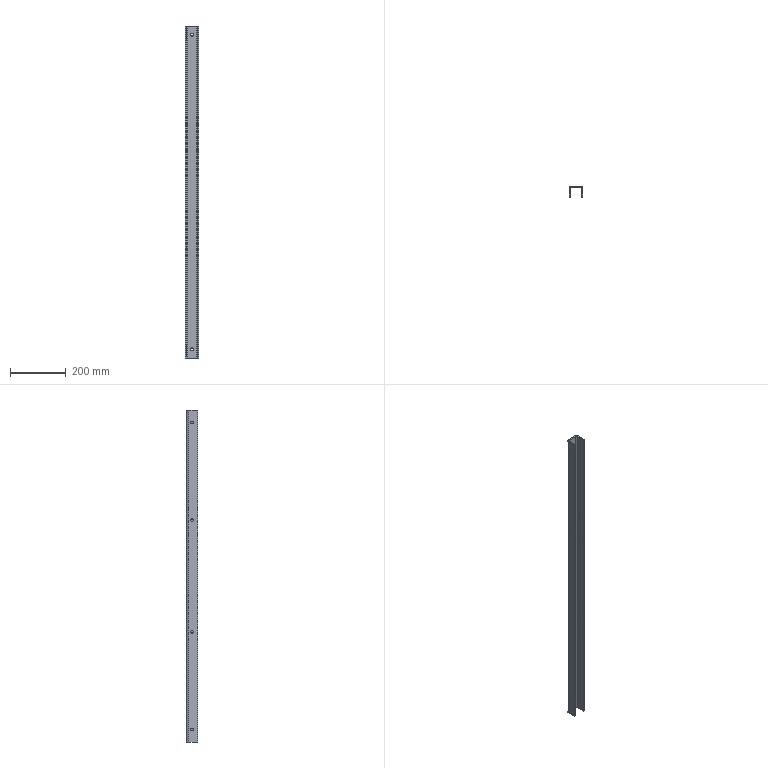Part | SolidWorks | features ICE 3, FlatPattern 1, SMBaseFlange 1, SheetMetal 1 | 1 solid | 42 faces | box 50 x 40 x 1190 mm | volume 552905 mm3 | cylinder 24 | plane 18 | commonest cylinder face diameters 11 x12 9 x8 8 x2 16 x2
STEP:
#1=CARTESIAN_POINT('',(-21.,-20.,554.5));
#2=VERTEX_POINT('',#1);
#3=CARTESIAN_POINT('',(-21.,-20.,545.5));
#4=VERTEX_POINT('',#3);
#5=CARTESIAN_POINT('',(-21.,-20.,550.));
#6=DIRECTION('',(1.,0.,0.));
#7=DIRECTION('',(0.,0.,1.));
#8=AXIS2_PLACEMENT_3D('',#5,#6,#7);
#9=CIRCLE('',#8,4.5);
#10=EDGE_CURVE('',#2,#4,#9,.T.);
#11=ORIENTED_EDGE('',*,*,#10,.T.);
#12=CARTESIAN_POINT('',(-25.,-20.,545.5));
#13=VERTEX_POINT('',#12);
#14=CARTESIAN_POINT('',(25.001,-20.,545.5));
#15=DIRECTION('',(-1.,0.,0.));
#16=VECTOR('',#15,1000.);
#17=LINE('',#14,#16);
#18=EDGE_CURVE('',#4,#13,#17,.T.);
#19=ORIENTED_EDGE('',*,*,#18,.T.);
#20=CARTESIAN_POINT('',(-25.,-20.,554.5));
#21=VERTEX_POINT('',#20);
#22=CARTESIAN_POINT('',(-25.,-20.,550.));
#23=DIRECTION('',(-1.,0.,0.));
#24=DIRECTION('',(0.,0.,1.));
#25=AXIS2_PLACEMENT_3D('',#22,#23,#24);
#26=CIRCLE('',#25,4.5);
#27=EDGE_CURVE('',#13,#21,#26,.T.);
#28=ORIENTED_EDGE('',*,*,#27,.T.);
#29=CARTESIAN_POINT('',(25.001,-20.,554.5));
#30=DIRECTION('',(-1.,0.,0.));
#31=VECTOR('',#30,1000.);
#32=LINE('',#29,#31);
#33=EDGE_CURVE('',#2,#21,#32,.T.);
#34=ORIENTED_EDGE('',*,*,#33,.F.);
#35=EDGE_LOOP('',(#11,#19,#28,#34));
#36=FACE_OUTER_BOUND('',#35,.T.);
#37=CARTESIAN_POINT('',(25.001,-20.,550.));
#38=DIRECTION('',(-1.,0.,0.));
#39=DIRECTION('',(0.,0.,1.));
#40=AXIS2_PLACEMENT_3D('',#37,#38,#39);
#41=CYLINDRICAL_SURFACE('',#40,4.5);
#42=ADVANCED_FACE('',(#36),#41,.F.);
#43=CARTESIAN_POINT('',(-21.,-20.,-545.5));
#44=VERTEX_POINT('',#43);
#45=CARTESIAN_POINT('',(-21.,-20.,-554.5));
#46=VERTEX_POINT('',#45);
#47=CARTESIAN_POINT('',(-21.,-20.,-550.));
#48=DIRECTION('',(1.,0.,0.));
#49=DIRECTION('',(0.,0.,1.));
#50=AXIS2_PLACEMENT_3D('',#47,#48,#49);
#51=CIRCLE('',#50,4.5);
#52=EDGE_CURVE('',#44,#46,#51,.T.);
#53=ORIENTED_EDGE('',*,*,#52,.T.);
#54=CARTESIAN_POINT('',(-25.,-20.,-554.5));
#55=VERTEX_POINT('',#54);
#56=CARTESIAN_POINT('',(25.001,-20.,-554.5));
#57=DIRECTION('',(-1.,0.,0.));
#58=VECTOR('',#57,1000.);
#59=LINE('',#56,#58);
#60=EDGE_CURVE('',#46,#55,#59,.T.);
#61=ORIENTED_EDGE('',*,*,#60,.T.);
#62=CARTESIAN_POINT('',(-25.,-20.,-545.5));
#63=VERTEX_POINT('',#62);
#64=CARTESIAN_POINT('',(-25.,-20.,-550.));
#65=DIRECTION('',(-1.,0.,0.));
#66=DIRECTION('',(0.,0.,-1.));
#67=AXIS2_PLACEMENT_3D('',#64,#65,#66);
#68=CIRCLE('',#67,4.5);
#69=EDGE_CURVE('',#55,#63,#68,.T.);
#70=ORIENTED_EDGE('',*,*,#69,.T.);
#71=CARTESIAN_POINT('',(25.001,-20.,-545.5));
#72=DIRECTION('',(-1.,0.,0.));
#73=VECTOR('',#72,1000.);
#74=LINE('',#71,#73);
#75=EDGE_CURVE('',#44,#63,#74,.T.);
#76=ORIENTED_EDGE('',*,*,#75,.F.);
#77=EDGE_LOOP('',(#53,#61,#70,#76));
#78=FACE_OUTER_BOUND('',#77,.T.);
#79=CARTESIAN_POINT('',(25.001,-20.,-550.));
#80=DIRECTION('',(-1.,0.,0.));
#81=DIRECTION('',(0.,0.,1.));
#82=AXIS2_PLACEMENT_3D('',#79,#80,#81);
#83=CYLINDRICAL_SURFACE('',#82,4.5);
#84=ADVANCED_FACE('',(#78),#83,.F.);
#85=CARTESIAN_POINT('',(-21.,-20.,-195.5));
#86=VERTEX_POINT('',#85);
#87=CARTESIAN_POINT('',(-21.,-20.,-204.5));
#88=VERTEX_POINT('',#87);
#89=CARTESIAN_POINT('',(-21.,-20.,-200.));
#90=DIRECTION('',(1.,0.,0.));
#91=DIRECTION('',(0.,0.,1.));
#92=AXIS2_PLACEMENT_3D('',#89,#90,#91);
#93=CIRCLE('',#92,4.5);
#94=EDGE_CURVE('',#86,#88,#93,.T.);
#95=ORIENTED_EDGE('',*,*,#94,.T.);
#96=CARTESIAN_POINT('',(-25.,-20.,-204.5));
#97=VERTEX_POINT('',#96);
#98=CARTESIAN_POINT('',(25.001,-20.,-204.5));
#99=DIRECTION('',(-1.,0.,0.));
#100=VECTOR('',#99,1000.);
#101=LINE('',#98,#100);
#102=EDGE_CURVE('',#88,#97,#101,.T.);
#103=ORIENTED_EDGE('',*,*,#102,.T.);
#104=CARTESIAN_POINT('',(-25.,-20.,-195.5));
#105=VERTEX_POINT('',#104);
#106=CARTESIAN_POINT('',(-25.,-20.,-200.));
#107=DIRECTION('',(-1.,0.,0.));
#108=DIRECTION('',(0.,0.,-1.));
#109=AXIS2_PLACEMENT_3D('',#106,#107,#108);
#110=CIRCLE('',#109,4.5);
#111=EDGE_CURVE('',#97,#105,#110,.T.);
#112=ORIENTED_EDGE('',*,*,#111,.T.);
#113=CARTESIAN_POINT('',(25.001,-20.,-195.5));
#114=DIRECTION('',(-1.,0.,0.));
#115=VECTOR('',#114,1000.);
#116=LINE('',#113,#115);
#117=EDGE_CURVE('',#86,#105,#116,.T.);
#118=ORIENTED_EDGE('',*,*,#117,.F.);
#119=EDGE_LOOP('',(#95,#103,#112,#118));
#120=FACE_OUTER_BOUND('',#119,.T.);
#121=CARTESIAN_POINT('',(25.001,-20.,-200.));
#122=DIRECTION('',(-1.,0.,0.));
#123=DIRECTION('',(0.,0.,1.));
#124=AXIS2_PLACEMENT_3D('',#121,#122,#123);
#125=CYLINDRICAL_SURFACE('',#124,4.5);
#126=ADVANCED_FACE('',(#120),#125,.F.);
#127=CARTESIAN_POINT('',(-21.,-20.,204.5));
#128=VERTEX_POINT('',#127);
#129=CARTESIAN_POINT('',(-21.,-20.,195.5));
#130=VERTEX_POINT('',#129);
#131=CARTESIAN_POINT('',(-21.,-20.,200.));
#132=DIRECTION('',(1.,0.,0.));
#133=DIRECTION('',(0.,0.,1.));
#134=AXIS2_PLACEMENT_3D('',#131,#132,#133);
#135=CIRCLE('',#134,4.5);
#136=EDGE_CURVE('',#128,#130,#135,.T.);
#137=ORIENTED_EDGE('',*,*,#136,.T.);
#138=CARTESIAN_POINT('',(-25.,-20.,195.5));
#139=VERTEX_POINT('',#138);
#140=CARTESIAN_POINT('',(25.001,-20.,195.5));
#141=DIRECTION('',(-1.,0.,0.));
#142=VECTOR('',#141,1000.);
#143=LINE('',#140,#142);
#144=EDGE_CURVE('',#130,#139,#143,.T.);
#145=ORIENTED_EDGE('',*,*,#144,.T.);
#146=CARTESIAN_POINT('',(-25.,-20.,204.5));
#147=VERTEX_POINT('',#146);
#148=CARTESIAN_POINT('',(-25.,-20.,200.));
#149=DIRECTION('',(-1.,0.,0.));
#150=DIRECTION('',(0.,0.,1.));
#151=AXIS2_PLACEMENT_3D('',#148,#149,#150);
#152=CIRCLE('',#151,4.5);
#153=EDGE_CURVE('',#139,#147,#152,.T.);
#154=ORIENTED_EDGE('',*,*,#153,.T.);
#155=CARTESIAN_POINT('',(25.001,-20.,204.5));
#156=DIRECTION('',(-1.,0.,0.));
#157=VECTOR('',#156,1000.);
#158=LINE('',#155,#157);
#159=EDGE_CURVE('',#128,#147,#158,.T.);
#160=ORIENTED_EDGE('',*,*,#159,.F.);
#161=EDGE_LOOP('',(#137,#145,#154,#160));
#162=FACE_OUTER_BOUND('',#161,.T.);
#163=CARTESIAN_POINT('',(25.001,-20.,200.));
#164=DIRECTION('',(-1.,0.,0.));
#165=DIRECTION('',(0.,0.,1.));
#166=AXIS2_PLACEMENT_3D('',#163,#164,#165);
#167=CYLINDRICAL_SURFACE('',#166,4.5);
#168=ADVANCED_FACE('',(#162),#167,.F.);
#169=CARTESIAN_POINT('',(21.,-20.,252.));
#170=VERTEX_POINT('',#169);
#171=CARTESIAN_POINT('',(21.,-20.,263.));
#172=VERTEX_POINT('',#171);
#173=CARTESIAN_POINT('',(21.,-20.,257.5));
#174=DIRECTION('',(-1.,0.,0.));
#175=DIRECTION('',(0.,0.,-1.));
#176=AXIS2_PLACEMENT_3D('',#173,#174,#175);
#177=CIRCLE('',#176,5.5);
#178=EDGE_CURVE('',#170,#172,#177,.T.);
#179=ORIENTED_EDGE('',*,*,#178,.T.);
#180=CARTESIAN_POINT('',(25.,-20.,263.));
#181=VERTEX_POINT('',#180);
#182=CARTESIAN_POINT('',(-25.001,-20.,263.));
#183=DIRECTION('',(1.,0.,0.));
#184=VECTOR('',#183,1000.);
#185=LINE('',#182,#184);
#186=EDGE_CURVE('',#172,#181,#185,.T.);
#187=ORIENTED_EDGE('',*,*,#186,.T.);
#188=CARTESIAN_POINT('',(25.,-20.,252.));
#189=VERTEX_POINT('',#188);
#190=CARTESIAN_POINT('',(25.,-20.,257.5));
#191=DIRECTION('',(1.,0.,0.));
#192=DIRECTION('',(0.,0.,-1.));
#193=AXIS2_PLACEMENT_3D('',#190,#191,#192);
#194=CIRCLE('',#193,5.5);
#195=EDGE_CURVE('',#181,#189,#194,.T.);
#196=ORIENTED_EDGE('',*,*,#195,.T.);
#197=CARTESIAN_POINT('',(-25.001,-20.,252.));
#198=DIRECTION('',(1.,0.,0.));
#199=VECTOR('',#198,1000.);
#200=LINE('',#197,#199);
#201=EDGE_CURVE('',#170,#189,#200,.T.);
#202=ORIENTED_EDGE('',*,*,#201,.F.);
#203=EDGE_LOOP('',(#179,#187,#196,#202));
#204=FACE_OUTER_BOUND('',#203,.T.);
#205=CARTESIAN_POINT('',(-25.001,-20.,257.5));
#206=DIRECTION('',(1.,0.,0.));
#207=DIRECTION('',(0.,0.,-1.));
#208=AXIS2_PLACEMENT_3D('',#205,#206,#207);
#209=CYLINDRICAL_SURFACE('',#208,5.5);
#210=ADVANCED_FACE('',(#204),#209,.F.);
#211=CARTESIAN_POINT('',(21.,-20.,147.));
#212=VERTEX_POINT('',#211);
#213=CARTESIAN_POINT('',(21.,-20.,158.));
#214=VERTEX_POINT('',#213);
#215=CARTESIAN_POINT('',(21.,-20.,152.5));
#216=DIRECTION('',(-1.,0.,0.));
#217=DIRECTION('',(0.,0.,-1.));
#218=AXIS2_PLACEMENT_3D('',#215,#216,#217);
#219=CIRCLE('',#218,5.5);
#220=EDGE_CURVE('',#212,#214,#219,.T.);
#221=ORIENTED_EDGE('',*,*,#220,.T.);
#222=CARTESIAN_POINT('',(25.,-20.,158.));
#223=VERTEX_POINT('',#222);
#224=CARTESIAN_POINT('',(-25.001,-20.,158.));
#225=DIRECTION('',(1.,0.,0.));
#226=VECTOR('',#225,1000.);
#227=LINE('',#224,#226);
#228=EDGE_CURVE('',#214,#223,#227,.T.);
#229=ORIENTED_EDGE('',*,*,#228,.T.);
#230=CARTESIAN_POINT('',(25.,-20.,147.));
#231=VERTEX_POINT('',#230);
#232=CARTESIAN_POINT('',(25.,-20.,152.5));
#233=DIRECTION('',(1.,0.,0.));
#234=DIRECTION('',(0.,0.,-1.));
#235=AXIS2_PLACEMENT_3D('',#232,#233,#234);
#236=CIRCLE('',#235,5.5);
#237=EDGE_CURVE('',#223,#231,#236,.T.);
#238=ORIENTED_EDGE('',*,*,#237,.T.);
#239=CARTESIAN_POINT('',(-25.001,-20.,147.));
#240=DIRECTION('',(1.,0.,0.));
#241=VECTOR('',#240,1000.);
#242=LINE('',#239,#241);
#243=EDGE_CURVE('',#212,#231,#242,.T.);
#244=ORIENTED_EDGE('',*,*,#243,.F.);
#245=EDGE_LOOP('',(#221,#229,#238,#244));
#246=FACE_OUTER_BOUND('',#245,.T.);
#247=CARTESIAN_POINT('',(-25.001,-20.,152.5));
#248=DIRECTION('',(1.,0.,0.));
#249=DIRECTION('',(0.,0.,-1.));
#250=AXIS2_PLACEMENT_3D('',#247,#248,#249);
#251=CYLINDRICAL_SURFACE('',#250,5.5);
#252=ADVANCED_FACE('',(#246),#251,.F.);
#253=CARTESIAN_POINT('',(21.,-20.,-158.));
#254=VERTEX_POINT('',#253);
#255=CARTESIAN_POINT('',(21.,-20.,-147.));
#256=VERTEX_POINT('',#255);
#257=CARTESIAN_POINT('',(21.,-20.,-152.5));
#258=DIRECTION('',(-1.,0.,0.));
#259=DIRECTION('',(0.,0.,-1.));
#260=AXIS2_PLACEMENT_3D('',#257,#258,#259);
#261=CIRCLE('',#260,5.5);
#262=EDGE_CURVE('',#254,#256,#261,.T.);
#263=ORIENTED_EDGE('',*,*,#262,.T.);
#264=CARTESIAN_POINT('',(25.,-20.,-147.));
#265=VERTEX_POINT('',#264);
#266=CARTESIAN_POINT('',(-25.001,-20.,-147.));
#267=DIRECTION('',(1.,0.,0.));
#268=VECTOR('',#267,1000.);
#269=LINE('',#266,#268);
#270=EDGE_CURVE('',#256,#265,#269,.T.);
#271=ORIENTED_EDGE('',*,*,#270,.T.);
#272=CARTESIAN_POINT('',(25.,-20.,-158.));
#273=VERTEX_POINT('',#272);
#274=CARTESIAN_POINT('',(25.,-20.,-152.5));
#275=DIRECTION('',(1.,0.,0.));
#276=DIRECTION('',(0.,0.,1.));
#277=AXIS2_PLACEMENT_3D('',#274,#275,#276);
#278=CIRCLE('',#277,5.5);
#279=EDGE_CURVE('',#265,#273,#278,.T.);
#280=ORIENTED_EDGE('',*,*,#279,.T.);
#281=CARTESIAN_POINT('',(-25.001,-20.,-158.));
#282=DIRECTION('',(1.,0.,0.));
#283=VECTOR('',#282,1000.);
#284=LINE('',#281,#283);
#285=EDGE_CURVE('',#254,#273,#284,.T.);
#286=ORIENTED_EDGE('',*,*,#285,.F.);
#287=EDGE_LOOP('',(#263,#271,#280,#286));
#288=FACE_OUTER_BOUND('',#287,.T.);
#289=CARTESIAN_POINT('',(-25.001,-20.,-152.5));
#290=DIRECTION('',(1.,0.,0.));
#291=DIRECTION('',(0.,0.,-1.));
#292=AXIS2_PLACEMENT_3D('',#289,#290,#291);
#293=CYLINDRICAL_SURFACE('',#292,5.5);
#294=ADVANCED_FACE('',(#288),#293,.F.);
#295=CARTESIAN_POINT('',(21.,-20.,-263.));
#296=VERTEX_POINT('',#295);
#297=CARTESIAN_POINT('',(21.,-20.,-252.));
#298=VERTEX_POINT('',#297);
#299=CARTESIAN_POINT('',(21.,-20.,-257.5));
#300=DIRECTION('',(-1.,0.,0.));
#301=DIRECTION('',(0.,0.,-1.));
#302=AXIS2_PLACEMENT_3D('',#299,#300,#301);
#303=CIRCLE('',#302,5.5);
#304=EDGE_CURVE('',#296,#298,#303,.T.);
#305=ORIENTED_EDGE('',*,*,#304,.T.);
#306=CARTESIAN_POINT('',(25.,-20.,-252.));
#307=VERTEX_POINT('',#306);
#308=CARTESIAN_POINT('',(-25.001,-20.,-252.));
#309=DIRECTION('',(1.,0.,0.));
#310=VECTOR('',#309,1000.);
#311=LINE('',#308,#310);
#312=EDGE_CURVE('',#298,#307,#311,.T.);
#313=ORIENTED_EDGE('',*,*,#312,.T.);
#314=CARTESIAN_POINT('',(25.,-20.,-263.));
#315=VERTEX_POINT('',#314);
#316=CARTESIAN_POINT('',(25.,-20.,-257.5));
#317=DIRECTION('',(1.,0.,0.));
#318=DIRECTION('',(0.,0.,1.));
#319=AXIS2_PLACEMENT_3D('',#316,#317,#318);
#320=CIRCLE('',#319,5.5);
#321=EDGE_CURVE('',#307,#315,#320,.T.);
#322=ORIENTED_EDGE('',*,*,#321,.T.);
#323=CARTESIAN_POINT('',(-25.001,-20.,-263.));
#324=DIRECTION('',(1.,0.,0.));
#325=VECTOR('',#324,1000.);
#326=LINE('',#323,#325);
#327=EDGE_CURVE('',#296,#315,#326,.T.);
#328=ORIENTED_EDGE('',*,*,#327,.F.);
#329=EDGE_LOOP('',(#305,#313,#322,#328));
#330=FACE_OUTER_BOUND('',#329,.T.);
#331=CARTESIAN_POINT('',(-25.001,-20.,-257.5));
#332=DIRECTION('',(1.,0.,0.));
#333=DIRECTION('',(0.,0.,-1.));
#334=AXIS2_PLACEMENT_3D('',#331,#332,#333);
#335=CYLINDRICAL_SURFACE('',#334,5.5);
#336=ADVANCED_FACE('',(#330),#335,.F.);
#337=CARTESIAN_POINT('',(5.5,-4.,564.));
#338=VERTEX_POINT('',#337);
#339=CARTESIAN_POINT('',(-5.5,-4.,564.));
#340=VERTEX_POINT('',#339);
#341=CARTESIAN_POINT('',(0.,-4.,564.));
#342=DIRECTION('',(0.,1.,0.));
#343=DIRECTION('',(0.,0.,1.));
#344=AXIS2_PLACEMENT_3D('',#341,#342,#343);
#345=CIRCLE('',#344,5.5);
#346=EDGE_CURVE('',#338,#340,#345,.T.);
#347=ORIENTED_EDGE('',*,*,#346,.F.);
#348=CARTESIAN_POINT('',(5.5,0.,564.));
#349=VERTEX_POINT('',#348);
#350=CARTESIAN_POINT('',(5.5,-40.,564.));
#351=DIRECTION('',(0.,1.,0.));
#352=VECTOR('',#351,1000.);
#353=LINE('',#350,#352);
#354=EDGE_CURVE('',#338,#349,#353,.T.);
#355=ORIENTED_EDGE('',*,*,#354,.T.);
#356=CARTESIAN_POINT('',(-5.5,0.,564.));
#357=VERTEX_POINT('',#356);
#358=CARTESIAN_POINT('',(0.,0.,564.));
#359=DIRECTION('',(0.,1.,0.));
#360=DIRECTION('',(-1.,0.,0.));
#361=AXIS2_PLACEMENT_3D('',#358,#359,#360);
#362=CIRCLE('',#361,5.5);
#363=EDGE_CURVE('',#349,#357,#362,.T.);
#364=ORIENTED_EDGE('',*,*,#363,.T.);
#365=CARTESIAN_POINT('',(-5.5,-40.,564.));
#366=DIRECTION('',(0.,1.,0.));
#367=VECTOR('',#366,1000.);
#368=LINE('',#365,#367);
#369=EDGE_CURVE('',#340,#357,#368,.T.);
#370=ORIENTED_EDGE('',*,*,#369,.F.);
#371=EDGE_LOOP('',(#347,#355,#364,#370));
#372=FACE_OUTER_BOUND('',#371,.T.);
#373=CARTESIAN_POINT('',(0.,-40.,564.));
#374=DIRECTION('',(0.,1.,0.));
#375=DIRECTION('',(-1.,0.,0.));
#376=AXIS2_PLACEMENT_3D('',#373,#374,#375);
#377=CYLINDRICAL_SURFACE('',#376,5.5);
#378=ADVANCED_FACE('',(#372),#377,.F.);
#379=CARTESIAN_POINT('',(5.5,-4.,-564.));
#380=VERTEX_POINT('',#379);
#381=CARTESIAN_POINT('',(-5.5,-4.,-564.));
#382=VERTEX_POINT('',#381);
#383=CARTESIAN_POINT('',(0.,-4.,-564.));
#384=DIRECTION('',(0.,1.,0.));
#385=DIRECTION('',(0.,0.,1.));
#386=AXIS2_PLACEMENT_3D('',#383,#384,#385);
#387=CIRCLE('',#386,5.5);
#388=EDGE_CURVE('',#380,#382,#387,.T.);
#389=ORIENTED_EDGE('',*,*,#388,.F.);
#390=CARTESIAN_POINT('',(5.5,0.,-564.));
#391=VERTEX_POINT('',#390);
#392=CARTESIAN_POINT('',(5.5,-40.,-564.));
#393=DIRECTION('',(0.,1.,0.));
#394=VECTOR('',#393,1000.);
#395=LINE('',#392,#394);
#396=EDGE_CURVE('',#380,#391,#395,.T.);
#397=ORIENTED_EDGE('',*,*,#396,.T.);
#398=CARTESIAN_POINT('',(-5.5,0.,-564.));
#399=VERTEX_POINT('',#398);
#400=CARTESIAN_POINT('',(0.,0.,-564.));
#401=DIRECTION('',(0.,1.,0.));
#402=DIRECTION('',(1.,0.,0.));
#403=AXIS2_PLACEMENT_3D('',#400,#401,#402);
#404=CIRCLE('',#403,5.5);
#405=EDGE_CURVE('',#391,#399,#404,.T.);
#406=ORIENTED_EDGE('',*,*,#405,.T.);
#407=CARTESIAN_POINT('',(-5.5,-40.,-564.));
#408=DIRECTION('',(0.,1.,0.));
#409=VECTOR('',#408,1000.);
#410=LINE('',#407,#409);
#411=EDGE_CURVE('',#382,#399,#410,.T.);
#412=ORIENTED_EDGE('',*,*,#411,.F.);
#413=EDGE_LOOP('',(#389,#397,#406,#412));
#414=FACE_OUTER_BOUND('',#413,.T.);
#415=CARTESIAN_POINT('',(0.,-40.,-564.));
#416=DIRECTION('',(0.,1.,0.));
#417=DIRECTION('',(-1.,0.,0.));
#418=AXIS2_PLACEMENT_3D('',#415,#416,#417);
#419=CYLINDRICAL_SURFACE('',#418,5.5);
#420=ADVANCED_FACE('',(#414),#419,.F.);
#421=CARTESIAN_POINT('',(-17.,0.,595.));
#422=VERTEX_POINT('',#421);
#423=CARTESIAN_POINT('',(-17.,-4.,595.));
#424=VERTEX_POINT('',#423);
#425=CARTESIAN_POINT('',(-17.,0.,595.));
#426=DIRECTION('',(0.,-1.,0.));
#427=VECTOR('',#426,1000.);
#428=LINE('',#425,#427);
#429=EDGE_CURVE('',#422,#424,#428,.T.);
#430=ORIENTED_EDGE('',*,*,#429,.F.);
#431=CARTESIAN_POINT('',(-25.,-8.,595.));
#432=VERTEX_POINT('',#431);
#433=CARTESIAN_POINT('',(-17.,-8.,595.));
#434=DIRECTION('',(0.,0.,-1.));
#435=DIRECTION('',(1.,0.,0.));
#436=AXIS2_PLACEMENT_3D('',#433,#434,#435);
#437=CIRCLE('',#436,8.);
#438=EDGE_CURVE('',#432,#422,#437,.T.);
#439=ORIENTED_EDGE('',*,*,#438,.F.);
#440=CARTESIAN_POINT('',(-21.,-8.,595.));
#441=VERTEX_POINT('',#440);
#442=CARTESIAN_POINT('',(-21.,-8.,595.));
#443=DIRECTION('',(-1.,0.,0.));
#444=VECTOR('',#443,1000.);
#445=LINE('',#442,#444);
#446=EDGE_CURVE('',#441,#432,#445,.T.);
#447=ORIENTED_EDGE('',*,*,#446,.F.);
#448=CARTESIAN_POINT('',(-17.,-8.,595.));
#449=DIRECTION('',(0.,0.,-1.));
#450=DIRECTION('',(1.,0.,0.));
#451=AXIS2_PLACEMENT_3D('',#448,#449,#450);
#452=CIRCLE('',#451,4.);
#453=EDGE_CURVE('',#441,#424,#452,.T.);
#454=ORIENTED_EDGE('',*,*,#453,.T.);
#455=EDGE_LOOP('',(#430,#439,#447,#454));
#456=FACE_OUTER_BOUND('',#455,.T.);
#457=CARTESIAN_POINT('',(-17.,0.,595.));
#458=DIRECTION('',(0.,0.,1.));
#459=DIRECTION('',(1.,0.,0.));
#460=AXIS2_PLACEMENT_3D('',#457,#458,#459);
#461=PLANE('',#460);
#462=ADVANCED_FACE('',(#456),#461,.T.);
#463=CARTESIAN_POINT('',(17.,0.,595.));
#464=VERTEX_POINT('',#463);
#465=CARTESIAN_POINT('',(-25.,0.,595.));
#466=DIRECTION('',(1.,0.,0.));
#467=VECTOR('',#466,1000.);
#468=LINE('',#465,#467);
#469=EDGE_CURVE('',#422,#464,#468,.T.);
#470=ORIENTED_EDGE('',*,*,#469,.F.);
#471=ORIENTED_EDGE('',*,*,#429,.T.);
#472=CARTESIAN_POINT('',(17.,-4.,595.));
#473=VERTEX_POINT('',#472);
#474=CARTESIAN_POINT('',(-25.,-4.,595.));
#475=DIRECTION('',(1.,0.,0.));
#476=VECTOR('',#475,1000.);
#477=LINE('',#474,#476);
#478=EDGE_CURVE('',#424,#473,#477,.T.);
#479=ORIENTED_EDGE('',*,*,#478,.T.);
#480=CARTESIAN_POINT('',(17.,-4.,595.));
#481=DIRECTION('',(0.,1.,0.));
#482=VECTOR('',#481,1000.);
#483=LINE('',#480,#482);
#484=EDGE_CURVE('',#473,#464,#483,.T.);
#485=ORIENTED_EDGE('',*,*,#484,.T.);
#486=EDGE_LOOP('',(#470,#471,#479,#485));
#487=FACE_OUTER_BOUND('',#486,.T.);
#488=CARTESIAN_POINT('',(-21.,-8.,595.));
#489=DIRECTION('',(0.,0.,1.));
#490=DIRECTION('',(1.,0.,0.));
#491=AXIS2_PLACEMENT_3D('',#488,#489,#490);
#492=PLANE('',#491);
#493=ADVANCED_FACE('',(#487),#492,.T.);
#494=CARTESIAN_POINT('',(-25.,-8.,-595.));
#495=VERTEX_POINT('',#494);
#496=CARTESIAN_POINT('',(-21.,-8.,-595.));
#497=VERTEX_POINT('',#496);
#498=CARTESIAN_POINT('',(-25.,-8.,-595.));
#499=DIRECTION('',(1.,0.,0.));
#500=VECTOR('',#499,1000.);
#501=LINE('',#498,#500);
#502=EDGE_CURVE('',#495,#497,#501,.T.);
#503=ORIENTED_EDGE('',*,*,#502,.F.);
#504=CARTESIAN_POINT('',(-17.,0.,-595.));
#505=VERTEX_POINT('',#504);
#506=CARTESIAN_POINT('',(-17.,-8.,-595.));
#507=DIRECTION('',(0.,0.,-1.));
#508=DIRECTION('',(1.,0.,0.));
#509=AXIS2_PLACEMENT_3D('',#506,#507,#508);
#510=CIRCLE('',#509,8.);
#511=EDGE_CURVE('',#495,#505,#510,.T.);
#512=ORIENTED_EDGE('',*,*,#511,.T.);
#513=CARTESIAN_POINT('',(-17.,-4.,-595.));
#514=VERTEX_POINT('',#513);
#515=CARTESIAN_POINT('',(-17.,-4.,-595.));
#516=DIRECTION('',(0.,1.,0.));
#517=VECTOR('',#516,1000.);
#518=LINE('',#515,#517);
#519=EDGE_CURVE('',#514,#505,#518,.T.);
#520=ORIENTED_EDGE('',*,*,#519,.F.);
#521=CARTESIAN_POINT('',(-17.,-8.,-595.));
#522=DIRECTION('',(0.,0.,-1.));
#523=DIRECTION('',(1.,0.,0.));
#524=AXIS2_PLACEMENT_3D('',#521,#522,#523);
#525=CIRCLE('',#524,4.);
#526=EDGE_CURVE('',#497,#514,#525,.T.);
#527=ORIENTED_EDGE('',*,*,#526,.F.);
#528=EDGE_LOOP('',(#503,#512,#520,#527));
#529=FACE_OUTER_BOUND('',#528,.T.);
#530=CARTESIAN_POINT('',(-25.,-8.,-595.));
#531=DIRECTION('',(0.,0.,-1.));
#532=DIRECTION('',(-1.,0.,0.));
#533=AXIS2_PLACEMENT_3D('',#530,#531,#532);
#534=PLANE('',#533);
#535=ADVANCED_FACE('',(#529),#534,.T.);
#536=CARTESIAN_POINT('',(-25.,-40.,-595.));
#537=VERTEX_POINT('',#536);
#538=CARTESIAN_POINT('',(-25.,-40.,-595.));
#539=DIRECTION('',(0.,1.,0.));
#540=VECTOR('',#539,1000.);
#541=LINE('',#538,#540);
#542=EDGE_CURVE('',#537,#495,#541,.T.);
#543=ORIENTED_EDGE('',*,*,#542,.T.);
#544=ORIENTED_EDGE('',*,*,#502,.T.);
#545=CARTESIAN_POINT('',(-21.,-40.,-595.));
#546=VERTEX_POINT('',#545);
#547=CARTESIAN_POINT('',(-21.,-40.,-595.));
#548=DIRECTION('',(0.,1.,0.));
#549=VECTOR('',#548,1000.);
#550=LINE('',#547,#549);
#551=EDGE_CURVE('',#546,#497,#550,.T.);
#552=ORIENTED_EDGE('',*,*,#551,.F.);
#553=CARTESIAN_POINT('',(-21.,-40.,-595.));
#554=DIRECTION('',(-1.,0.,0.));
#555=VECTOR('',#554,1000.);
#556=LINE('',#553,#555);
#557=EDGE_CURVE('',#546,#537,#556,.T.);
#558=ORIENTED_EDGE('',*,*,#557,.T.);
#559=EDGE_LOOP('',(#543,#544,#552,#558));
#560=FACE_OUTER_BOUND('',#559,.T.);
#561=CARTESIAN_POINT('',(-17.,-4.,-595.));
#562=DIRECTION('',(0.,0.,-1.));
#563=DIRECTION('',(-1.,0.,0.));
#564=AXIS2_PLACEMENT_3D('',#561,#562,#563);
#565=PLANE('',#564);
#566=ADVANCED_FACE('',(#560),#565,.T.);
#567=CARTESIAN_POINT('',(25.,-8.,595.));
#568=VERTEX_POINT('',#567);
#569=CARTESIAN_POINT('',(21.,-8.,595.));
#570=VERTEX_POINT('',#569);
#571=CARTESIAN_POINT('',(25.,-8.,595.));
#572=DIRECTION('',(-1.,0.,0.));
#573=VECTOR('',#572,1000.);
#574=LINE('',#571,#573);
#575=EDGE_CURVE('',#568,#570,#574,.T.);
#576=ORIENTED_EDGE('',*,*,#575,.F.);
#577=CARTESIAN_POINT('',(17.,-8.,595.));
#578=DIRECTION('',(0.,0.,-1.));
#579=DIRECTION('',(1.,0.,0.));
#580=AXIS2_PLACEMENT_3D('',#577,#578,#579);
#581=CIRCLE('',#580,8.);
#582=EDGE_CURVE('',#464,#568,#581,.T.);
#583=ORIENTED_EDGE('',*,*,#582,.F.);
#584=ORIENTED_EDGE('',*,*,#484,.F.);
#585=CARTESIAN_POINT('',(17.,-8.,595.));
#586=DIRECTION('',(0.,0.,-1.));
#587=DIRECTION('',(1.,0.,0.));
#588=AXIS2_PLACEMENT_3D('',#585,#586,#587);
#589=CIRCLE('',#588,4.);
#590=EDGE_CURVE('',#473,#570,#589,.T.);
#591=ORIENTED_EDGE('',*,*,#590,.T.);
#592=EDGE_LOOP('',(#576,#583,#584,#591));
#593=FACE_OUTER_BOUND('',#592,.T.);
#594=CARTESIAN_POINT('',(25.,-8.,595.));
#595=DIRECTION('',(0.,0.,1.));
#596=DIRECTION('',(1.,0.,0.));
#597=AXIS2_PLACEMENT_3D('',#594,#595,#596);
#598=PLANE('',#597);
#599=ADVANCED_FACE('',(#593),#598,.T.);
#600=CARTESIAN_POINT('',(25.,-40.,595.));
#601=VERTEX_POINT('',#600);
#602=CARTESIAN_POINT('',(25.,0.,595.));
#603=DIRECTION('',(0.,-1.,0.));
#604=VECTOR('',#603,1000.);
#605=LINE('',#602,#604);
#606=EDGE_CURVE('',#568,#601,#605,.T.);
#607=ORIENTED_EDGE('',*,*,#606,.F.);
#608=ORIENTED_EDGE('',*,*,#575,.T.);
#609=CARTESIAN_POINT('',(21.,-40.,595.));
#610=VERTEX_POINT('',#609);
#611=CARTESIAN_POINT('',(21.,0.,595.));
#612=DIRECTION('',(0.,-1.,0.));
#613=VECTOR('',#612,1000.);
#614=LINE('',#611,#613);
#615=EDGE_CURVE('',#570,#610,#614,.T.);
#616=ORIENTED_EDGE('',*,*,#615,.T.);
#617=CARTESIAN_POINT('',(25.,-40.,595.));
#618=DIRECTION('',(-1.,0.,0.));
#619=VECTOR('',#618,1000.);
#620=LINE('',#617,#619);
#621=EDGE_CURVE('',#601,#610,#620,.T.);
#622=ORIENTED_EDGE('',*,*,#621,.F.);
#623=EDGE_LOOP('',(#607,#608,#616,#622));
#624=FACE_OUTER_BOUND('',#623,.T.);
#625=CARTESIAN_POINT('',(17.,-4.,595.));
#626=DIRECTION('',(0.,0.,1.));
#627=DIRECTION('',(1.,0.,0.));
#628=AXIS2_PLACEMENT_3D('',#625,#626,#627);
#629=PLANE('',#628);
#630=ADVANCED_FACE('',(#624),#629,.T.);
#631=CARTESIAN_POINT('',(17.,0.,-595.));
#632=VERTEX_POINT('',#631);
#633=CARTESIAN_POINT('',(17.,-4.,-595.));
#634=VERTEX_POINT('',#633);
#635=CARTESIAN_POINT('',(17.,0.,-595.));
#636=DIRECTION('',(0.,-1.,0.));
#637=VECTOR('',#636,1000.);
#638=LINE('',#635,#637);
#639=EDGE_CURVE('',#632,#634,#638,.T.);
#640=ORIENTED_EDGE('',*,*,#639,.F.);
#641=CARTESIAN_POINT('',(25.,-8.,-595.));
#642=VERTEX_POINT('',#641);
#643=CARTESIAN_POINT('',(17.,-8.,-595.));
#644=DIRECTION('',(0.,0.,-1.));
#645=DIRECTION('',(1.,0.,0.));
#646=AXIS2_PLACEMENT_3D('',#643,#644,#645);
#647=CIRCLE('',#646,8.);
#648=EDGE_CURVE('',#632,#642,#647,.T.);
#649=ORIENTED_EDGE('',*,*,#648,.T.);
#650=CARTESIAN_POINT('',(21.,-8.,-595.));
#651=VERTEX_POINT('',#650);
#652=CARTESIAN_POINT('',(21.,-8.,-595.));
#653=DIRECTION('',(1.,0.,0.));
#654=VECTOR('',#653,1000.);
#655=LINE('',#652,#654);
#656=EDGE_CURVE('',#651,#642,#655,.T.);
#657=ORIENTED_EDGE('',*,*,#656,.F.);
#658=CARTESIAN_POINT('',(17.,-8.,-595.));
#659=DIRECTION('',(0.,0.,-1.));
#660=DIRECTION('',(1.,0.,0.));
#661=AXIS2_PLACEMENT_3D('',#658,#659,#660);
#662=CIRCLE('',#661,4.);
#663=EDGE_CURVE('',#634,#651,#662,.T.);
#664=ORIENTED_EDGE('',*,*,#663,.F.);
#665=EDGE_LOOP('',(#640,#649,#657,#664));
#666=FACE_OUTER_BOUND('',#665,.T.);
#667=CARTESIAN_POINT('',(17.,0.,-595.));
#668=DIRECTION('',(0.,0.,-1.));
#669=DIRECTION('',(-1.,0.,0.));
#670=AXIS2_PLACEMENT_3D('',#667,#668,#669);
#671=PLANE('',#670);
#672=ADVANCED_FACE('',(#666),#671,.T.);
#673=CARTESIAN_POINT('',(-25.,0.,-595.));
#674=DIRECTION('',(1.,0.,0.));
#675=VECTOR('',#674,1000.);
#676=LINE('',#673,#675);
#677=EDGE_CURVE('',#505,#632,#676,.T.);
#678=ORIENTED_EDGE('',*,*,#677,.T.);
#679=ORIENTED_EDGE('',*,*,#639,.T.);
#680=CARTESIAN_POINT('',(-25.,-4.,-595.));
#681=DIRECTION('',(1.,0.,0.));
#682=VECTOR('',#681,1000.);
#683=LINE('',#680,#682);
#684=EDGE_CURVE('',#514,#634,#683,.T.);
#685=ORIENTED_EDGE('',*,*,#684,.F.);
#686=ORIENTED_EDGE('',*,*,#519,.T.);
#687=EDGE_LOOP('',(#678,#679,#685,#686));
#688=FACE_OUTER_BOUND('',#687,.T.);
#689=CARTESIAN_POINT('',(21.,-8.,-595.));
#690=DIRECTION('',(0.,0.,-1.));
#691=DIRECTION('',(-1.,0.,0.));
#692=AXIS2_PLACEMENT_3D('',#689,#690,#691);
#693=PLANE('',#692);
#694=ADVANCED_FACE('',(#688),#693,.T.);
#695=ORIENTED_EDGE('',*,*,#178,.F.);
#696=CARTESIAN_POINT('',(21.,-20.,257.5));
#697=DIRECTION('',(-1.,0.,0.));
#698=DIRECTION('',(0.,0.,-1.));
#699=AXIS2_PLACEMENT_3D('',#696,#697,#698);
#700=CIRCLE('',#699,5.5);
#701=EDGE_CURVE('',#172,#170,#700,.T.);
#702=ORIENTED_EDGE('',*,*,#701,.F.);
#703=EDGE_LOOP('',(#695,#702));
#704=FACE_BOUND('',#703,.T.);
#705=ORIENTED_EDGE('',*,*,#220,.F.);
#706=CARTESIAN_POINT('',(21.,-20.,152.5));
#707=DIRECTION('',(-1.,0.,0.));
#708=DIRECTION('',(0.,0.,-1.));
#709=AXIS2_PLACEMENT_3D('',#706,#707,#708);
#710=CIRCLE('',#709,5.5);
#711=EDGE_CURVE('',#214,#212,#710,.T.);
#712=ORIENTED_EDGE('',*,*,#711,.F.);
#713=EDGE_LOOP('',(#705,#712));
#714=FACE_BOUND('',#713,.T.);
#715=ORIENTED_EDGE('',*,*,#262,.F.);
#716=CARTESIAN_POINT('',(21.,-20.,-152.5));
#717=DIRECTION('',(-1.,0.,0.));
#718=DIRECTION('',(0.,0.,-1.));
#719=AXIS2_PLACEMENT_3D('',#716,#717,#718);
#720=CIRCLE('',#719,5.5);
#721=EDGE_CURVE('',#256,#254,#720,.T.);
#722=ORIENTED_EDGE('',*,*,#721,.F.);
#723=EDGE_LOOP('',(#715,#722));
#724=FACE_BOUND('',#723,.T.);
#725=ORIENTED_EDGE('',*,*,#304,.F.);
#726=CARTESIAN_POINT('',(21.,-20.,-257.5));
#727=DIRECTION('',(-1.,0.,0.));
#728=DIRECTION('',(0.,0.,-1.));
#729=AXIS2_PLACEMENT_3D('',#726,#727,#728);
#730=CIRCLE('',#729,5.5);
#731=EDGE_CURVE('',#298,#296,#730,.T.);
#732=ORIENTED_EDGE('',*,*,#731,.F.);
#733=EDGE_LOOP('',(#725,#732));
#734=FACE_BOUND('',#733,.T.);
#735=CARTESIAN_POINT('',(21.,-40.,-595.));
#736=VERTEX_POINT('',#735);
#737=CARTESIAN_POINT('',(21.,0.,-595.));
#738=DIRECTION('',(0.,-1.,0.));
#739=VECTOR('',#738,1000.);
#740=LINE('',#737,#739);
#741=EDGE_CURVE('',#651,#736,#740,.T.);
#742=ORIENTED_EDGE('',*,*,#741,.T.);
#743=CARTESIAN_POINT('',(21.,-40.,595.));
#744=DIRECTION('',(0.,0.,-1.));
#745=VECTOR('',#744,1000.);
#746=LINE('',#743,#745);
#747=EDGE_CURVE('',#610,#736,#746,.T.);
#748=ORIENTED_EDGE('',*,*,#747,.F.);
#749=ORIENTED_EDGE('',*,*,#615,.F.);
#750=CARTESIAN_POINT('',(21.,-8.,595.));
#751=DIRECTION('',(0.,0.,-1.));
#752=VECTOR('',#751,1000.);
#753=LINE('',#750,#752);
#754=EDGE_CURVE('',#570,#651,#753,.T.);
#755=ORIENTED_EDGE('',*,*,#754,.T.);
#756=EDGE_LOOP('',(#742,#748,#749,#755));
#757=FACE_OUTER_BOUND('',#756,.T.);
#758=CARTESIAN_POINT('',(21.,0.,595.));
#759=DIRECTION('',(1.,0.,0.));
#760=DIRECTION('',(0.,0.,-1.));
#761=AXIS2_PLACEMENT_3D('',#758,#759,#760);
#762=PLANE('',#761);
#763=ADVANCED_FACE('',(#704,#714,#724,#734,#757),#762,.F.);
#764=CARTESIAN_POINT('',(25.,-40.,-595.));
#765=VERTEX_POINT('',#764);
#766=CARTESIAN_POINT('',(25.,-40.,-595.));
#767=DIRECTION('',(-1.,0.,0.));
#768=VECTOR('',#767,1000.);
#769=LINE('',#766,#768);
#770=EDGE_CURVE('',#765,#736,#769,.T.);
#771=ORIENTED_EDGE('',*,*,#770,.F.);
#772=CARTESIAN_POINT('',(25.,-40.,595.));
#773=DIRECTION('',(0.,0.,-1.));
#774=VECTOR('',#773,1000.);
#775=LINE('',#772,#774);
#776=EDGE_CURVE('',#601,#765,#775,.T.);
#777=ORIENTED_EDGE('',*,*,#776,.F.);
#778=ORIENTED_EDGE('',*,*,#621,.T.);
#779=ORIENTED_EDGE('',*,*,#747,.T.);
#780=EDGE_LOOP('',(#771,#777,#778,#779));
#781=FACE_OUTER_BOUND('',#780,.T.);
#782=CARTESIAN_POINT('',(25.,-40.,595.));
#783=DIRECTION('',(0.,-1.,0.));
#784=DIRECTION('',(0.,0.,-1.));
#785=AXIS2_PLACEMENT_3D('',#782,#783,#784);
#786=PLANE('',#785);
#787=ADVANCED_FACE('',(#781),#786,.T.);
#788=CARTESIAN_POINT('',(25.,-20.,257.5));
#789=DIRECTION('',(1.,0.,0.));
#790=DIRECTION('',(0.,0.,-1.));
#791=AXIS2_PLACEMENT_3D('',#788,#789,#790);
#792=CIRCLE('',#791,5.5);
#793=EDGE_CURVE('',#189,#181,#792,.T.);
#794=ORIENTED_EDGE('',*,*,#793,.F.);
#795=ORIENTED_EDGE('',*,*,#195,.F.);
#796=EDGE_LOOP('',(#794,#795));
#797=FACE_BOUND('',#796,.T.);
#798=CARTESIAN_POINT('',(25.,-20.,152.5));
#799=DIRECTION('',(1.,0.,0.));
#800=DIRECTION('',(0.,0.,-1.));
#801=AXIS2_PLACEMENT_3D('',#798,#799,#800);
#802=CIRCLE('',#801,5.5);
#803=EDGE_CURVE('',#231,#223,#802,.T.);
#804=ORIENTED_EDGE('',*,*,#803,.F.);
#805=ORIENTED_EDGE('',*,*,#237,.F.);
#806=EDGE_LOOP('',(#804,#805));
#807=FACE_BOUND('',#806,.T.);
#808=CARTESIAN_POINT('',(25.,-20.,-152.5));
#809=DIRECTION('',(1.,0.,0.));
#810=DIRECTION('',(0.,0.,1.));
#811=AXIS2_PLACEMENT_3D('',#808,#809,#810);
#812=CIRCLE('',#811,5.5);
#813=EDGE_CURVE('',#273,#265,#812,.T.);
#814=ORIENTED_EDGE('',*,*,#813,.F.);
#815=ORIENTED_EDGE('',*,*,#279,.F.);
#816=EDGE_LOOP('',(#814,#815));
#817=FACE_BOUND('',#816,.T.);
#818=CARTESIAN_POINT('',(25.,-20.,-257.5));
#819=DIRECTION('',(1.,0.,0.));
#820=DIRECTION('',(0.,0.,1.));
#821=AXIS2_PLACEMENT_3D('',#818,#819,#820);
#822=CIRCLE('',#821,5.5);
#823=EDGE_CURVE('',#315,#307,#822,.T.);
#824=ORIENTED_EDGE('',*,*,#823,.F.);
#825=ORIENTED_EDGE('',*,*,#321,.F.);
#826=EDGE_LOOP('',(#824,#825));
#827=FACE_BOUND('',#826,.T.);
#828=CARTESIAN_POINT('',(25.,0.,-595.));
#829=DIRECTION('',(0.,-1.,0.));
#830=VECTOR('',#829,1000.);
#831=LINE('',#828,#830);
#832=EDGE_CURVE('',#642,#765,#831,.T.);
#833=ORIENTED_EDGE('',*,*,#832,.F.);
#834=CARTESIAN_POINT('',(25.,-8.,595.));
#835=DIRECTION('',(0.,0.,-1.));
#836=VECTOR('',#835,1000.);
#837=LINE('',#834,#836);
#838=EDGE_CURVE('',#568,#642,#837,.T.);
#839=ORIENTED_EDGE('',*,*,#838,.F.);
#840=ORIENTED_EDGE('',*,*,#606,.T.);
#841=ORIENTED_EDGE('',*,*,#776,.T.);
#842=EDGE_LOOP('',(#833,#839,#840,#841));
#843=FACE_OUTER_BOUND('',#842,.T.);
#844=CARTESIAN_POINT('',(25.,0.,595.));
#845=DIRECTION('',(1.,0.,0.));
#846=DIRECTION('',(0.,0.,-1.));
#847=AXIS2_PLACEMENT_3D('',#844,#845,#846);
#848=PLANE('',#847);
#849=ADVANCED_FACE('',(#797,#807,#817,#827,#843),#848,.T.);
#850=ORIENTED_EDGE('',*,*,#648,.F.);
#851=CARTESIAN_POINT('',(17.,0.,595.));
#852=DIRECTION('',(0.,0.,-1.));
#853=VECTOR('',#852,1000.);
#854=LINE('',#851,#853);
#855=EDGE_CURVE('',#464,#632,#854,.T.);
#856=ORIENTED_EDGE('',*,*,#855,.F.);
#857=ORIENTED_EDGE('',*,*,#582,.T.);
#858=ORIENTED_EDGE('',*,*,#838,.T.);
#859=EDGE_LOOP('',(#850,#856,#857,#858));
#860=FACE_OUTER_BOUND('',#859,.T.);
#861=CARTESIAN_POINT('',(17.,-8.,595.));
#862=DIRECTION('',(0.,0.,-1.));
#863=DIRECTION('',(-1.,0.,0.));
#864=AXIS2_PLACEMENT_3D('',#861,#862,#863);
#865=CYLINDRICAL_SURFACE('',#864,8.);
#866=ADVANCED_FACE('',(#860),#865,.T.);
#867=CARTESIAN_POINT('',(0.,0.,564.));
#868=DIRECTION('',(0.,1.,0.));
#869=DIRECTION('',(-1.,0.,0.));
#870=AXIS2_PLACEMENT_3D('',#867,#868,#869);
#871=CIRCLE('',#870,5.5);
#872=EDGE_CURVE('',#357,#349,#871,.T.);
#873=ORIENTED_EDGE('',*,*,#872,.F.);
#874=ORIENTED_EDGE('',*,*,#363,.F.);
#875=EDGE_LOOP('',(#873,#874));
#876=FACE_BOUND('',#875,.T.);
#877=CARTESIAN_POINT('',(0.,0.,-564.));
#878=DIRECTION('',(0.,1.,0.));
#879=DIRECTION('',(1.,0.,0.));
#880=AXIS2_PLACEMENT_3D('',#877,#878,#879);
#881=CIRCLE('',#880,5.5);
#882=EDGE_CURVE('',#399,#391,#881,.T.);
#883=ORIENTED_EDGE('',*,*,#882,.F.);
#884=ORIENTED_EDGE('',*,*,#405,.F.);
#885=EDGE_LOOP('',(#883,#884));
#886=FACE_BOUND('',#885,.T.);
#887=ORIENTED_EDGE('',*,*,#677,.F.);
#888=CARTESIAN_POINT('',(-17.,0.,595.));
#889=DIRECTION('',(0.,0.,-1.));
#890=VECTOR('',#889,1000.);
#891=LINE('',#888,#890);
#892=EDGE_CURVE('',#422,#505,#891,.T.);
#893=ORIENTED_EDGE('',*,*,#892,.F.);
#894=ORIENTED_EDGE('',*,*,#469,.T.);
#895=ORIENTED_EDGE('',*,*,#855,.T.);
#896=EDGE_LOOP('',(#887,#893,#894,#895));
#897=FACE_OUTER_BOUND('',#896,.T.);
#898=CARTESIAN_POINT('',(-25.,0.,595.));
#899=DIRECTION('',(0.,1.,0.));
#900=DIRECTION('',(0.,0.,1.));
#901=AXIS2_PLACEMENT_3D('',#898,#899,#900);
#902=PLANE('',#901);
#903=ADVANCED_FACE('',(#876,#886,#897),#902,.T.);
#904=ORIENTED_EDGE('',*,*,#511,.F.);
#905=CARTESIAN_POINT('',(-25.,-8.,595.));
#906=DIRECTION('',(0.,0.,-1.));
#907=VECTOR('',#906,1000.);
#908=LINE('',#905,#907);
#909=EDGE_CURVE('',#432,#495,#908,.T.);
#910=ORIENTED_EDGE('',*,*,#909,.F.);
#911=ORIENTED_EDGE('',*,*,#438,.T.);
#912=ORIENTED_EDGE('',*,*,#892,.T.);
#913=EDGE_LOOP('',(#904,#910,#911,#912));
#914=FACE_OUTER_BOUND('',#913,.T.);
#915=CARTESIAN_POINT('',(-17.,-8.,595.));
#916=DIRECTION('',(0.,0.,-1.));
#917=DIRECTION('',(-1.,0.,0.));
#918=AXIS2_PLACEMENT_3D('',#915,#916,#917);
#919=CYLINDRICAL_SURFACE('',#918,8.);
#920=ADVANCED_FACE('',(#914),#919,.T.);
#921=CARTESIAN_POINT('',(-25.,-20.,550.));
#922=DIRECTION('',(-1.,0.,0.));
#923=DIRECTION('',(0.,0.,1.));
#924=AXIS2_PLACEMENT_3D('',#921,#922,#923);
#925=CIRCLE('',#924,4.5);
#926=EDGE_CURVE('',#21,#13,#925,.T.);
#927=ORIENTED_EDGE('',*,*,#926,.F.);
#928=ORIENTED_EDGE('',*,*,#27,.F.);
#929=EDGE_LOOP('',(#927,#928));
#930=FACE_BOUND('',#929,.T.);
#931=CARTESIAN_POINT('',(-25.,-20.,-550.));
#932=DIRECTION('',(-1.,0.,0.));
#933=DIRECTION('',(0.,0.,-1.));
#934=AXIS2_PLACEMENT_3D('',#931,#932,#933);
#935=CIRCLE('',#934,4.5);
#936=EDGE_CURVE('',#63,#55,#935,.T.);
#937=ORIENTED_EDGE('',*,*,#936,.F.);
#938=ORIENTED_EDGE('',*,*,#69,.F.);
#939=EDGE_LOOP('',(#937,#938));
#940=FACE_BOUND('',#939,.T.);
#941=CARTESIAN_POINT('',(-25.,-20.,-200.));
#942=DIRECTION('',(-1.,0.,0.));
#943=DIRECTION('',(0.,0.,-1.));
#944=AXIS2_PLACEMENT_3D('',#941,#942,#943);
#945=CIRCLE('',#944,4.5);
#946=EDGE_CURVE('',#105,#97,#945,.T.);
#947=ORIENTED_EDGE('',*,*,#946,.F.);
#948=ORIENTED_EDGE('',*,*,#111,.F.);
#949=EDGE_LOOP('',(#947,#948));
#950=FACE_BOUND('',#949,.T.);
#951=CARTESIAN_POINT('',(-25.,-20.,200.));
#952=DIRECTION('',(-1.,0.,0.));
#953=DIRECTION('',(0.,0.,1.));
#954=AXIS2_PLACEMENT_3D('',#951,#952,#953);
#955=CIRCLE('',#954,4.5);
#956=EDGE_CURVE('',#147,#139,#955,.T.);
#957=ORIENTED_EDGE('',*,*,#956,.F.);
#958=ORIENTED_EDGE('',*,*,#153,.F.);
#959=EDGE_LOOP('',(#957,#958));
#960=FACE_BOUND('',#959,.T.);
#961=ORIENTED_EDGE('',*,*,#542,.F.);
#962=CARTESIAN_POINT('',(-25.,-40.,595.));
#963=VERTEX_POINT('',#962);
#964=CARTESIAN_POINT('',(-25.,-40.,595.));
#965=DIRECTION('',(0.,0.,-1.));
#966=VECTOR('',#965,1000.);
#967=LINE('',#964,#966);
#968=EDGE_CURVE('',#963,#537,#967,.T.);
#969=ORIENTED_EDGE('',*,*,#968,.F.);
#970=CARTESIAN_POINT('',(-25.,-40.,595.));
#971=DIRECTION('',(0.,1.,0.));
#972=VECTOR('',#971,1000.);
#973=LINE('',#970,#972);
#974=EDGE_CURVE('',#963,#432,#973,.T.);
#975=ORIENTED_EDGE('',*,*,#974,.T.);
#976=ORIENTED_EDGE('',*,*,#909,.T.);
#977=EDGE_LOOP('',(#961,#969,#975,#976));
#978=FACE_OUTER_BOUND('',#977,.T.);
#979=CARTESIAN_POINT('',(-25.,-40.,595.));
#980=DIRECTION('',(-1.,0.,0.));
#981=DIRECTION('',(0.,0.,1.));
#982=AXIS2_PLACEMENT_3D('',#979,#980,#981);
#983=PLANE('',#982);
#984=ADVANCED_FACE('',(#930,#940,#950,#960,#978),#983,.T.);
#985=ORIENTED_EDGE('',*,*,#557,.F.);
#986=CARTESIAN_POINT('',(-21.,-40.,595.));
#987=VERTEX_POINT('',#986);
#988=CARTESIAN_POINT('',(-21.,-40.,595.));
#989=DIRECTION('',(0.,0.,-1.));
#990=VECTOR('',#989,1000.);
#991=LINE('',#988,#990);
#992=EDGE_CURVE('',#987,#546,#991,.T.);
#993=ORIENTED_EDGE('',*,*,#992,.F.);
#994=CARTESIAN_POINT('',(-21.,-40.,595.));
#995=DIRECTION('',(-1.,0.,0.));
#996=VECTOR('',#995,1000.);
#997=LINE('',#994,#996);
#998=EDGE_CURVE('',#987,#963,#997,.T.);
#999=ORIENTED_EDGE('',*,*,#998,.T.);
#1000=ORIENTED_EDGE('',*,*,#968,.T.);
#1001=EDGE_LOOP('',(#985,#993,#999,#1000));
#1002=FACE_OUTER_BOUND('',#1001,.T.);
#1003=CARTESIAN_POINT('',(-21.,-40.,595.));
#1004=DIRECTION('',(0.,-1.,0.));
#1005=DIRECTION('',(0.,0.,-1.));
#1006=AXIS2_PLACEMENT_3D('',#1003,#1004,#1005);
#1007=PLANE('',#1006);
#1008=ADVANCED_FACE('',(#1002),#1007,.T.);
#1009=ORIENTED_EDGE('',*,*,#10,.F.);
#1010=CARTESIAN_POINT('',(-21.,-20.,550.));
#1011=DIRECTION('',(1.,0.,0.));
#1012=DIRECTION('',(0.,0.,1.));
#1013=AXIS2_PLACEMENT_3D('',#1010,#1011,#1012);
#1014=CIRCLE('',#1013,4.5);
#1015=EDGE_CURVE('',#4,#2,#1014,.T.);
#1016=ORIENTED_EDGE('',*,*,#1015,.F.);
#1017=EDGE_LOOP('',(#1009,#1016));
#1018=FACE_BOUND('',#1017,.T.);
#1019=ORIENTED_EDGE('',*,*,#52,.F.);
#1020=CARTESIAN_POINT('',(-21.,-20.,-550.));
#1021=DIRECTION('',(1.,0.,0.));
#1022=DIRECTION('',(0.,0.,1.));
#1023=AXIS2_PLACEMENT_3D('',#1020,#1021,#1022);
#1024=CIRCLE('',#1023,4.5);
#1025=EDGE_CURVE('',#46,#44,#1024,.T.);
#1026=ORIENTED_EDGE('',*,*,#1025,.F.);
#1027=EDGE_LOOP('',(#1019,#1026));
#1028=FACE_BOUND('',#1027,.T.);
#1029=ORIENTED_EDGE('',*,*,#94,.F.);
#1030=CARTESIAN_POINT('',(-21.,-20.,-200.));
#1031=DIRECTION('',(1.,0.,0.));
#1032=DIRECTION('',(0.,0.,1.));
#1033=AXIS2_PLACEMENT_3D('',#1030,#1031,#1032);
#1034=CIRCLE('',#1033,4.5);
#1035=EDGE_CURVE('',#88,#86,#1034,.T.);
#1036=ORIENTED_EDGE('',*,*,#1035,.F.);
#1037=EDGE_LOOP('',(#1029,#1036));
#1038=FACE_BOUND('',#1037,.T.);
#1039=ORIENTED_EDGE('',*,*,#136,.F.);
#1040=CARTESIAN_POINT('',(-21.,-20.,200.));
#1041=DIRECTION('',(1.,0.,0.));
#1042=DIRECTION('',(0.,0.,1.));
#1043=AXIS2_PLACEMENT_3D('',#1040,#1041,#1042);
#1044=CIRCLE('',#1043,4.5);
#1045=EDGE_CURVE('',#130,#128,#1044,.T.);
#1046=ORIENTED_EDGE('',*,*,#1045,.F.);
#1047=EDGE_LOOP('',(#1039,#1046));
#1048=FACE_BOUND('',#1047,.T.);
#1049=ORIENTED_EDGE('',*,*,#551,.T.);
#1050=CARTESIAN_POINT('',(-21.,-8.,595.));
#1051=DIRECTION('',(0.,0.,-1.));
#1052=VECTOR('',#1051,1000.);
#1053=LINE('',#1050,#1052);
#1054=EDGE_CURVE('',#441,#497,#1053,.T.);
#1055=ORIENTED_EDGE('',*,*,#1054,.F.);
#1056=CARTESIAN_POINT('',(-21.,-40.,595.));
#1057=DIRECTION('',(0.,1.,0.));
#1058=VECTOR('',#1057,1000.);
#1059=LINE('',#1056,#1058);
#1060=EDGE_CURVE('',#987,#441,#1059,.T.);
#1061=ORIENTED_EDGE('',*,*,#1060,.F.);
#1062=ORIENTED_EDGE('',*,*,#992,.T.);
#1063=EDGE_LOOP('',(#1049,#1055,#1061,#1062));
#1064=FACE_OUTER_BOUND('',#1063,.T.);
#1065=CARTESIAN_POINT('',(-21.,-40.,595.));
#1066=DIRECTION('',(-1.,0.,0.));
#1067=DIRECTION('',(0.,0.,1.));
#1068=AXIS2_PLACEMENT_3D('',#1065,#1066,#1067);
#1069=PLANE('',#1068);
#1070=ADVANCED_FACE('',(#1018,#1028,#1038,#1048,#1064),#1069,.F.);
#1071=ORIENTED_EDGE('',*,*,#526,.T.);
#1072=CARTESIAN_POINT('',(-17.,-4.,595.));
#1073=DIRECTION('',(0.,0.,-1.));
#1074=VECTOR('',#1073,1000.);
#1075=LINE('',#1072,#1074);
#1076=EDGE_CURVE('',#424,#514,#1075,.T.);
#1077=ORIENTED_EDGE('',*,*,#1076,.F.);
#1078=ORIENTED_EDGE('',*,*,#453,.F.);
#1079=ORIENTED_EDGE('',*,*,#1054,.T.);
#1080=EDGE_LOOP('',(#1071,#1077,#1078,#1079));
#1081=FACE_OUTER_BOUND('',#1080,.T.);
#1082=CARTESIAN_POINT('',(-17.,-8.,595.));
#1083=DIRECTION('',(0.,0.,-1.));
#1084=DIRECTION('',(-1.,0.,0.));
#1085=AXIS2_PLACEMENT_3D('',#1082,#1083,#1084);
#1086=CYLINDRICAL_SURFACE('',#1085,4.);
#1087=ADVANCED_FACE('',(#1081),#1086,.F.);
#1088=CARTESIAN_POINT('',(0.,-4.,564.));
#1089=DIRECTION('',(0.,1.,0.));
#1090=DIRECTION('',(0.,0.,1.));
#1091=AXIS2_PLACEMENT_3D('',#1088,#1089,#1090);
#1092=CIRCLE('',#1091,5.5);
#1093=EDGE_CURVE('',#340,#338,#1092,.T.);
#1094=ORIENTED_EDGE('',*,*,#1093,.T.);
#1095=ORIENTED_EDGE('',*,*,#346,.T.);
#1096=EDGE_LOOP('',(#1094,#1095));
#1097=FACE_BOUND('',#1096,.T.);
#1098=CARTESIAN_POINT('',(0.,-4.,-564.));
#1099=DIRECTION('',(0.,1.,0.));
#1100=DIRECTION('',(0.,0.,1.));
#1101=AXIS2_PLACEMENT_3D('',#1098,#1099,#1100);
#1102=CIRCLE('',#1101,5.5);
#1103=EDGE_CURVE('',#382,#380,#1102,.T.);
#1104=ORIENTED_EDGE('',*,*,#1103,.T.);
#1105=ORIENTED_EDGE('',*,*,#388,.T.);
#1106=EDGE_LOOP('',(#1104,#1105));
#1107=FACE_BOUND('',#1106,.T.);
#1108=ORIENTED_EDGE('',*,*,#684,.T.);
#1109=CARTESIAN_POINT('',(17.,-4.,595.));
#1110=DIRECTION('',(0.,0.,-1.));
#1111=VECTOR('',#1110,1000.);
#1112=LINE('',#1109,#1111);
#1113=EDGE_CURVE('',#473,#634,#1112,.T.);
#1114=ORIENTED_EDGE('',*,*,#1113,.F.);
#1115=ORIENTED_EDGE('',*,*,#478,.F.);
#1116=ORIENTED_EDGE('',*,*,#1076,.T.);
#1117=EDGE_LOOP('',(#1108,#1114,#1115,#1116));
#1118=FACE_OUTER_BOUND('',#1117,.T.);
#1119=CARTESIAN_POINT('',(-25.,-4.,595.));
#1120=DIRECTION('',(0.,1.,0.));
#1121=DIRECTION('',(0.,0.,1.));
#1122=AXIS2_PLACEMENT_3D('',#1119,#1120,#1121);
#1123=PLANE('',#1122);
#1124=ADVANCED_FACE('',(#1097,#1107,#1118),#1123,.F.);
#1125=ORIENTED_EDGE('',*,*,#663,.T.);
#1126=ORIENTED_EDGE('',*,*,#754,.F.);
#1127=ORIENTED_EDGE('',*,*,#590,.F.);
#1128=ORIENTED_EDGE('',*,*,#1113,.T.);
#1129=EDGE_LOOP('',(#1125,#1126,#1127,#1128));
#1130=FACE_OUTER_BOUND('',#1129,.T.);
#1131=CARTESIAN_POINT('',(17.,-8.,595.));
#1132=DIRECTION('',(0.,0.,-1.));
#1133=DIRECTION('',(-1.,0.,0.));
#1134=AXIS2_PLACEMENT_3D('',#1131,#1132,#1133);
#1135=CYLINDRICAL_SURFACE('',#1134,4.);
#1136=ADVANCED_FACE('',(#1130),#1135,.F.);
#1137=ORIENTED_EDGE('',*,*,#1060,.T.);
#1138=ORIENTED_EDGE('',*,*,#446,.T.);
#1139=ORIENTED_EDGE('',*,*,#974,.F.);
#1140=ORIENTED_EDGE('',*,*,#998,.F.);
#1141=EDGE_LOOP('',(#1137,#1138,#1139,#1140));
#1142=FACE_OUTER_BOUND('',#1141,.T.);
#1143=CARTESIAN_POINT('',(17.,-8.,595.));
#1144=DIRECTION('',(0.,0.,1.));
#1145=DIRECTION('',(1.,0.,0.));
#1146=AXIS2_PLACEMENT_3D('',#1143,#1144,#1145);
#1147=PLANE('',#1146);
#1148=ADVANCED_FACE('',(#1142),#1147,.T.);
#1149=ORIENTED_EDGE('',*,*,#741,.F.);
#1150=ORIENTED_EDGE('',*,*,#656,.T.);
#1151=ORIENTED_EDGE('',*,*,#832,.T.);
#1152=ORIENTED_EDGE('',*,*,#770,.T.);
#1153=EDGE_LOOP('',(#1149,#1150,#1151,#1152));
#1154=FACE_OUTER_BOUND('',#1153,.T.);
#1155=CARTESIAN_POINT('',(17.,-8.,-595.));
#1156=DIRECTION('',(0.,0.,1.));
#1157=DIRECTION('',(1.,0.,0.));
#1158=AXIS2_PLACEMENT_3D('',#1155,#1156,#1157);
#1159=PLANE('',#1158);
#1160=ADVANCED_FACE('',(#1154),#1159,.F.);
#1161=ORIENTED_EDGE('',*,*,#396,.F.);
#1162=ORIENTED_EDGE('',*,*,#1103,.F.);
#1163=ORIENTED_EDGE('',*,*,#411,.T.);
#1164=ORIENTED_EDGE('',*,*,#882,.T.);
#1165=EDGE_LOOP('',(#1161,#1162,#1163,#1164));
#1166=FACE_OUTER_BOUND('',#1165,.T.);
#1167=CARTESIAN_POINT('',(0.,-40.,-564.));
#1168=DIRECTION('',(0.,1.,0.));
#1169=DIRECTION('',(-1.,0.,0.));
#1170=AXIS2_PLACEMENT_3D('',#1167,#1168,#1169);
#1171=CYLINDRICAL_SURFACE('',#1170,5.5);
#1172=ADVANCED_FACE('',(#1166),#1171,.F.);
#1173=ORIENTED_EDGE('',*,*,#354,.F.);
#1174=ORIENTED_EDGE('',*,*,#1093,.F.);
#1175=ORIENTED_EDGE('',*,*,#369,.T.);
#1176=ORIENTED_EDGE('',*,*,#872,.T.);
#1177=EDGE_LOOP('',(#1173,#1174,#1175,#1176));
#1178=FACE_OUTER_BOUND('',#1177,.T.);
#1179=CARTESIAN_POINT('',(0.,-40.,564.));
#1180=DIRECTION('',(0.,1.,0.));
#1181=DIRECTION('',(-1.,0.,0.));
#1182=AXIS2_PLACEMENT_3D('',#1179,#1180,#1181);
#1183=CYLINDRICAL_SURFACE('',#1182,5.5);
#1184=ADVANCED_FACE('',(#1178),#1183,.F.);
#1185=ORIENTED_EDGE('',*,*,#312,.F.);
#1186=ORIENTED_EDGE('',*,*,#731,.T.);
#1187=ORIENTED_EDGE('',*,*,#327,.T.);
#1188=ORIENTED_EDGE('',*,*,#823,.T.);
#1189=EDGE_LOOP('',(#1185,#1186,#1187,#1188));
#1190=FACE_OUTER_BOUND('',#1189,.T.);
#1191=CARTESIAN_POINT('',(-25.001,-20.,-257.5));
#1192=DIRECTION('',(1.,0.,0.));
#1193=DIRECTION('',(0.,0.,-1.));
#1194=AXIS2_PLACEMENT_3D('',#1191,#1192,#1193);
#1195=CYLINDRICAL_SURFACE('',#1194,5.5);
#1196=ADVANCED_FACE('',(#1190),#1195,.F.);
#1197=ORIENTED_EDGE('',*,*,#270,.F.);
#1198=ORIENTED_EDGE('',*,*,#721,.T.);
#1199=ORIENTED_EDGE('',*,*,#285,.T.);
#1200=ORIENTED_EDGE('',*,*,#813,.T.);
#1201=EDGE_LOOP('',(#1197,#1198,#1199,#1200));
#1202=FACE_OUTER_BOUND('',#1201,.T.);
#1203=CARTESIAN_POINT('',(-25.001,-20.,-152.5));
#1204=DIRECTION('',(1.,0.,0.));
#1205=DIRECTION('',(0.,0.,-1.));
#1206=AXIS2_PLACEMENT_3D('',#1203,#1204,#1205);
#1207=CYLINDRICAL_SURFACE('',#1206,5.5);
#1208=ADVANCED_FACE('',(#1202),#1207,.F.);
#1209=ORIENTED_EDGE('',*,*,#228,.F.);
#1210=ORIENTED_EDGE('',*,*,#711,.T.);
#1211=ORIENTED_EDGE('',*,*,#243,.T.);
#1212=ORIENTED_EDGE('',*,*,#803,.T.);
#1213=EDGE_LOOP('',(#1209,#1210,#1211,#1212));
#1214=FACE_OUTER_BOUND('',#1213,.T.);
#1215=CARTESIAN_POINT('',(-25.001,-20.,152.5));
#1216=DIRECTION('',(1.,0.,0.));
#1217=DIRECTION('',(0.,0.,-1.));
#1218=AXIS2_PLACEMENT_3D('',#1215,#1216,#1217);
#1219=CYLINDRICAL_SURFACE('',#1218,5.5);
#1220=ADVANCED_FACE('',(#1214),#1219,.F.);
#1221=ORIENTED_EDGE('',*,*,#186,.F.);
#1222=ORIENTED_EDGE('',*,*,#701,.T.);
#1223=ORIENTED_EDGE('',*,*,#201,.T.);
#1224=ORIENTED_EDGE('',*,*,#793,.T.);
#1225=EDGE_LOOP('',(#1221,#1222,#1223,#1224));
#1226=FACE_OUTER_BOUND('',#1225,.T.);
#1227=CARTESIAN_POINT('',(-25.001,-20.,257.5));
#1228=DIRECTION('',(1.,0.,0.));
#1229=DIRECTION('',(0.,0.,-1.));
#1230=AXIS2_PLACEMENT_3D('',#1227,#1228,#1229);
#1231=CYLINDRICAL_SURFACE('',#1230,5.5);
#1232=ADVANCED_FACE('',(#1226),#1231,.F.);
#1233=ORIENTED_EDGE('',*,*,#144,.F.);
#1234=ORIENTED_EDGE('',*,*,#1045,.T.);
#1235=ORIENTED_EDGE('',*,*,#159,.T.);
#1236=ORIENTED_EDGE('',*,*,#956,.T.);
#1237=EDGE_LOOP('',(#1233,#1234,#1235,#1236));
#1238=FACE_OUTER_BOUND('',#1237,.T.);
#1239=CARTESIAN_POINT('',(25.001,-20.,200.));
#1240=DIRECTION('',(-1.,0.,0.));
#1241=DIRECTION('',(0.,0.,1.));
#1242=AXIS2_PLACEMENT_3D('',#1239,#1240,#1241);
#1243=CYLINDRICAL_SURFACE('',#1242,4.5);
#1244=ADVANCED_FACE('',(#1238),#1243,.F.);
#1245=ORIENTED_EDGE('',*,*,#102,.F.);
#1246=ORIENTED_EDGE('',*,*,#1035,.T.);
#1247=ORIENTED_EDGE('',*,*,#117,.T.);
#1248=ORIENTED_EDGE('',*,*,#946,.T.);
#1249=EDGE_LOOP('',(#1245,#1246,#1247,#1248));
#1250=FACE_OUTER_BOUND('',#1249,.T.);
#1251=CARTESIAN_POINT('',(25.001,-20.,-200.));
#1252=DIRECTION('',(-1.,0.,0.));
#1253=DIRECTION('',(0.,0.,1.));
#1254=AXIS2_PLACEMENT_3D('',#1251,#1252,#1253);
#1255=CYLINDRICAL_SURFACE('',#1254,4.5);
#1256=ADVANCED_FACE('',(#1250),#1255,.F.);
#1257=ORIENTED_EDGE('',*,*,#60,.F.);
#1258=ORIENTED_EDGE('',*,*,#1025,.T.);
#1259=ORIENTED_EDGE('',*,*,#75,.T.);
#1260=ORIENTED_EDGE('',*,*,#936,.T.);
#1261=EDGE_LOOP('',(#1257,#1258,#1259,#1260));
#1262=FACE_OUTER_BOUND('',#1261,.T.);
#1263=CARTESIAN_POINT('',(25.001,-20.,-550.));
#1264=DIRECTION('',(-1.,0.,0.));
#1265=DIRECTION('',(0.,0.,1.));
#1266=AXIS2_PLACEMENT_3D('',#1263,#1264,#1265);
#1267=CYLINDRICAL_SURFACE('',#1266,4.5);
#1268=ADVANCED_FACE('',(#1262),#1267,.F.);
#1269=ORIENTED_EDGE('',*,*,#18,.F.);
#1270=ORIENTED_EDGE('',*,*,#1015,.T.);
#1271=ORIENTED_EDGE('',*,*,#33,.T.);
#1272=ORIENTED_EDGE('',*,*,#926,.T.);
#1273=EDGE_LOOP('',(#1269,#1270,#1271,#1272));
#1274=FACE_OUTER_BOUND('',#1273,.T.);
#1275=CARTESIAN_POINT('',(25.001,-20.,550.));
#1276=DIRECTION('',(-1.,0.,0.));
#1277=DIRECTION('',(0.,0.,1.));
#1278=AXIS2_PLACEMENT_3D('',#1275,#1276,#1277);
#1279=CYLINDRICAL_SURFACE('',#1278,4.5);
#1280=ADVANCED_FACE('',(#1274),#1279,.F.);
#1281=CLOSED_SHELL('',(#42,#84,#126,#168,#210,#252,#294,#336,#378,#420,#462,#493,#535,#566,#599,#630,#672,#694,#763,#787,#849,#866,#903,#920,#984,#1008,#1070,#1087,#1124,#1136,#1148,#1160,#1172,#1184,#1196,#1208,#1220,#1232,#1244,#1256,#1268,#1280));
#1282=MANIFOLD_SOLID_BREP('',#1281);
#1283=CARTESIAN_POINT('',(0.,0.,0.));
#1284=DIRECTION('',(0.,0.,1.));
#1285=DIRECTION('',(1.,0.,0.));
#1286=AXIS2_PLACEMENT_3D('',#1283,#1284,#1285);
#1287=(LENGTH_UNIT()NAMED_UNIT(*)SI_UNIT(.MILLI.,.METRE.));
#1288=UNCERTAINTY_MEASURE_WITH_UNIT(LENGTH_MEASURE(0.00001),#1287,'','');
#1289=(NAMED_UNIT(*)PLANE_ANGLE_UNIT()SI_UNIT($,.RADIAN.));
#1290=(NAMED_UNIT(*)SI_UNIT($,.STERADIAN.)SOLID_ANGLE_UNIT());
#1291=(GEOMETRIC_REPRESENTATION_CONTEXT(3)GLOBAL_UNCERTAINTY_ASSIGNED_CONTEXT((#1288))GLOBAL_UNIT_ASSIGNED_CONTEXT((#1287,#1289,#1290))REPRESENTATION_CONTEXT('',''));
#1292=ADVANCED_BREP_SHAPE_REPRESENTATION('',(#1282,#1286),#1291);